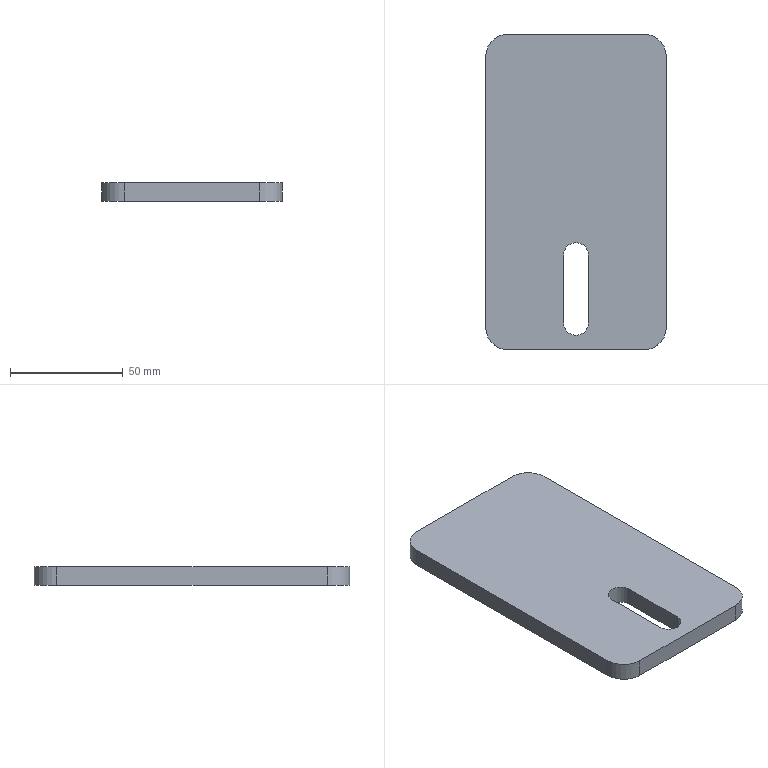Part | SolidWorks | features Extrusion 1, ICE 1 | 1 solid | 14 faces | box 80 x 140 x 8 mm | volume 85513 mm3 | plane 8 | cylinder 6 | commonest cylinder face diameters 20 x4 11 x2
STEP:
#1=CARTESIAN_POINT('',(70.,0.,0.));
#2=VERTEX_POINT('',#1);
#3=CARTESIAN_POINT('',(80.,10.,0.));
#4=VERTEX_POINT('',#3);
#5=CARTESIAN_POINT('',(70.,10.,0.));
#6=DIRECTION('',(0.,0.,1.));
#7=DIRECTION('',(-1.,0.,0.));
#8=AXIS2_PLACEMENT_3D('',#5,#6,#7);
#9=CIRCLE('',#8,10.);
#10=EDGE_CURVE('',#2,#4,#9,.T.);
#11=ORIENTED_EDGE('',*,*,#10,.T.);
#12=CARTESIAN_POINT('',(80.,10.,8.));
#13=VERTEX_POINT('',#12);
#14=CARTESIAN_POINT('',(80.,10.,8.));
#15=DIRECTION('',(0.,0.,-1.));
#16=VECTOR('',#15,1000.);
#17=LINE('',#14,#16);
#18=EDGE_CURVE('',#13,#4,#17,.T.);
#19=ORIENTED_EDGE('',*,*,#18,.F.);
#20=CARTESIAN_POINT('',(70.,0.,8.));
#21=VERTEX_POINT('',#20);
#22=CARTESIAN_POINT('',(70.,10.,8.));
#23=DIRECTION('',(0.,0.,1.));
#24=DIRECTION('',(-1.,0.,0.));
#25=AXIS2_PLACEMENT_3D('',#22,#23,#24);
#26=CIRCLE('',#25,10.);
#27=EDGE_CURVE('',#21,#13,#26,.T.);
#28=ORIENTED_EDGE('',*,*,#27,.F.);
#29=CARTESIAN_POINT('',(70.,0.,8.));
#30=DIRECTION('',(0.,0.,-1.));
#31=VECTOR('',#30,1000.);
#32=LINE('',#29,#31);
#33=EDGE_CURVE('',#21,#2,#32,.T.);
#34=ORIENTED_EDGE('',*,*,#33,.T.);
#35=EDGE_LOOP('',(#11,#19,#28,#34));
#36=FACE_OUTER_BOUND('',#35,.T.);
#37=CARTESIAN_POINT('',(70.,10.,8.));
#38=DIRECTION('',(0.,0.,-1.));
#39=DIRECTION('',(-1.,0.,0.));
#40=AXIS2_PLACEMENT_3D('',#37,#38,#39);
#41=CYLINDRICAL_SURFACE('',#40,10.);
#42=ADVANCED_FACE('',(#36),#41,.T.);
#43=CARTESIAN_POINT('',(80.,130.,0.));
#44=VERTEX_POINT('',#43);
#45=CARTESIAN_POINT('',(80.,10.,0.));
#46=DIRECTION('',(0.,1.,0.));
#47=VECTOR('',#46,1000.);
#48=LINE('',#45,#47);
#49=EDGE_CURVE('',#4,#44,#48,.T.);
#50=ORIENTED_EDGE('',*,*,#49,.T.);
#51=CARTESIAN_POINT('',(80.,130.,8.));
#52=VERTEX_POINT('',#51);
#53=CARTESIAN_POINT('',(80.,130.,8.));
#54=DIRECTION('',(0.,0.,-1.));
#55=VECTOR('',#54,1000.);
#56=LINE('',#53,#55);
#57=EDGE_CURVE('',#52,#44,#56,.T.);
#58=ORIENTED_EDGE('',*,*,#57,.F.);
#59=CARTESIAN_POINT('',(80.,10.,8.));
#60=DIRECTION('',(0.,1.,0.));
#61=VECTOR('',#60,1000.);
#62=LINE('',#59,#61);
#63=EDGE_CURVE('',#13,#52,#62,.T.);
#64=ORIENTED_EDGE('',*,*,#63,.F.);
#65=ORIENTED_EDGE('',*,*,#18,.T.);
#66=EDGE_LOOP('',(#50,#58,#64,#65));
#67=FACE_OUTER_BOUND('',#66,.T.);
#68=CARTESIAN_POINT('',(80.,10.,8.));
#69=DIRECTION('',(-1.,0.,0.));
#70=DIRECTION('',(0.,0.,1.));
#71=AXIS2_PLACEMENT_3D('',#68,#69,#70);
#72=PLANE('',#71);
#73=ADVANCED_FACE('',(#67),#72,.F.);
#74=CARTESIAN_POINT('',(70.,140.,0.));
#75=VERTEX_POINT('',#74);
#76=CARTESIAN_POINT('',(70.,130.,0.));
#77=DIRECTION('',(0.,0.,1.));
#78=DIRECTION('',(1.,0.,0.));
#79=AXIS2_PLACEMENT_3D('',#76,#77,#78);
#80=CIRCLE('',#79,10.);
#81=EDGE_CURVE('',#44,#75,#80,.T.);
#82=ORIENTED_EDGE('',*,*,#81,.T.);
#83=CARTESIAN_POINT('',(70.,140.,8.));
#84=VERTEX_POINT('',#83);
#85=CARTESIAN_POINT('',(70.,140.,8.));
#86=DIRECTION('',(0.,0.,-1.));
#87=VECTOR('',#86,1000.);
#88=LINE('',#85,#87);
#89=EDGE_CURVE('',#84,#75,#88,.T.);
#90=ORIENTED_EDGE('',*,*,#89,.F.);
#91=CARTESIAN_POINT('',(70.,130.,8.));
#92=DIRECTION('',(0.,0.,1.));
#93=DIRECTION('',(1.,0.,0.));
#94=AXIS2_PLACEMENT_3D('',#91,#92,#93);
#95=CIRCLE('',#94,10.);
#96=EDGE_CURVE('',#52,#84,#95,.T.);
#97=ORIENTED_EDGE('',*,*,#96,.F.);
#98=ORIENTED_EDGE('',*,*,#57,.T.);
#99=EDGE_LOOP('',(#82,#90,#97,#98));
#100=FACE_OUTER_BOUND('',#99,.T.);
#101=CARTESIAN_POINT('',(70.,130.,8.));
#102=DIRECTION('',(0.,0.,-1.));
#103=DIRECTION('',(-1.,0.,0.));
#104=AXIS2_PLACEMENT_3D('',#101,#102,#103);
#105=CYLINDRICAL_SURFACE('',#104,10.);
#106=ADVANCED_FACE('',(#100),#105,.T.);
#107=CARTESIAN_POINT('',(10.,140.,0.));
#108=VERTEX_POINT('',#107);
#109=CARTESIAN_POINT('',(10.,140.,0.));
#110=DIRECTION('',(-1.,0.,0.));
#111=VECTOR('',#110,1000.);
#112=LINE('',#109,#111);
#113=EDGE_CURVE('',#75,#108,#112,.T.);
#114=ORIENTED_EDGE('',*,*,#113,.T.);
#115=CARTESIAN_POINT('',(10.,140.,8.));
#116=VERTEX_POINT('',#115);
#117=CARTESIAN_POINT('',(10.,140.,8.));
#118=DIRECTION('',(0.,0.,-1.));
#119=VECTOR('',#118,1000.);
#120=LINE('',#117,#119);
#121=EDGE_CURVE('',#116,#108,#120,.T.);
#122=ORIENTED_EDGE('',*,*,#121,.F.);
#123=CARTESIAN_POINT('',(10.,140.,8.));
#124=DIRECTION('',(-1.,0.,0.));
#125=VECTOR('',#124,1000.);
#126=LINE('',#123,#125);
#127=EDGE_CURVE('',#84,#116,#126,.T.);
#128=ORIENTED_EDGE('',*,*,#127,.F.);
#129=ORIENTED_EDGE('',*,*,#89,.T.);
#130=EDGE_LOOP('',(#114,#122,#128,#129));
#131=FACE_OUTER_BOUND('',#130,.T.);
#132=CARTESIAN_POINT('',(10.,140.,8.));
#133=DIRECTION('',(0.,-1.,0.));
#134=DIRECTION('',(0.,0.,-1.));
#135=AXIS2_PLACEMENT_3D('',#132,#133,#134);
#136=PLANE('',#135);
#137=ADVANCED_FACE('',(#131),#136,.F.);
#138=CARTESIAN_POINT('',(0.,130.,0.));
#139=VERTEX_POINT('',#138);
#140=CARTESIAN_POINT('',(10.,130.,0.));
#141=DIRECTION('',(0.,0.,1.));
#142=DIRECTION('',(-1.,0.,0.));
#143=AXIS2_PLACEMENT_3D('',#140,#141,#142);
#144=CIRCLE('',#143,10.);
#145=EDGE_CURVE('',#108,#139,#144,.T.);
#146=ORIENTED_EDGE('',*,*,#145,.T.);
#147=CARTESIAN_POINT('',(0.,130.,8.));
#148=VERTEX_POINT('',#147);
#149=CARTESIAN_POINT('',(0.,130.,8.));
#150=DIRECTION('',(0.,0.,-1.));
#151=VECTOR('',#150,1000.);
#152=LINE('',#149,#151);
#153=EDGE_CURVE('',#148,#139,#152,.T.);
#154=ORIENTED_EDGE('',*,*,#153,.F.);
#155=CARTESIAN_POINT('',(10.,130.,8.));
#156=DIRECTION('',(0.,0.,1.));
#157=DIRECTION('',(-1.,0.,0.));
#158=AXIS2_PLACEMENT_3D('',#155,#156,#157);
#159=CIRCLE('',#158,10.);
#160=EDGE_CURVE('',#116,#148,#159,.T.);
#161=ORIENTED_EDGE('',*,*,#160,.F.);
#162=ORIENTED_EDGE('',*,*,#121,.T.);
#163=EDGE_LOOP('',(#146,#154,#161,#162));
#164=FACE_OUTER_BOUND('',#163,.T.);
#165=CARTESIAN_POINT('',(10.,130.,8.));
#166=DIRECTION('',(0.,0.,-1.));
#167=DIRECTION('',(-1.,0.,0.));
#168=AXIS2_PLACEMENT_3D('',#165,#166,#167);
#169=CYLINDRICAL_SURFACE('',#168,10.);
#170=ADVANCED_FACE('',(#164),#169,.T.);
#171=CARTESIAN_POINT('',(0.,10.,0.));
#172=VERTEX_POINT('',#171);
#173=CARTESIAN_POINT('',(0.,10.,0.));
#174=DIRECTION('',(0.,-1.,0.));
#175=VECTOR('',#174,1000.);
#176=LINE('',#173,#175);
#177=EDGE_CURVE('',#139,#172,#176,.T.);
#178=ORIENTED_EDGE('',*,*,#177,.T.);
#179=CARTESIAN_POINT('',(0.,10.,8.));
#180=VERTEX_POINT('',#179);
#181=CARTESIAN_POINT('',(0.,10.,8.));
#182=DIRECTION('',(0.,0.,-1.));
#183=VECTOR('',#182,1000.);
#184=LINE('',#181,#183);
#185=EDGE_CURVE('',#180,#172,#184,.T.);
#186=ORIENTED_EDGE('',*,*,#185,.F.);
#187=CARTESIAN_POINT('',(0.,10.,8.));
#188=DIRECTION('',(0.,-1.,0.));
#189=VECTOR('',#188,1000.);
#190=LINE('',#187,#189);
#191=EDGE_CURVE('',#148,#180,#190,.T.);
#192=ORIENTED_EDGE('',*,*,#191,.F.);
#193=ORIENTED_EDGE('',*,*,#153,.T.);
#194=EDGE_LOOP('',(#178,#186,#192,#193));
#195=FACE_OUTER_BOUND('',#194,.T.);
#196=CARTESIAN_POINT('',(0.,10.,8.));
#197=DIRECTION('',(1.,0.,0.));
#198=DIRECTION('',(0.,0.,-1.));
#199=AXIS2_PLACEMENT_3D('',#196,#197,#198);
#200=PLANE('',#199);
#201=ADVANCED_FACE('',(#195),#200,.F.);
#202=CARTESIAN_POINT('',(10.,0.,0.));
#203=VERTEX_POINT('',#202);
#204=CARTESIAN_POINT('',(10.,10.,0.));
#205=DIRECTION('',(0.,0.,1.));
#206=DIRECTION('',(-1.,0.,0.));
#207=AXIS2_PLACEMENT_3D('',#204,#205,#206);
#208=CIRCLE('',#207,10.);
#209=EDGE_CURVE('',#172,#203,#208,.T.);
#210=ORIENTED_EDGE('',*,*,#209,.T.);
#211=CARTESIAN_POINT('',(10.,0.,8.));
#212=VERTEX_POINT('',#211);
#213=CARTESIAN_POINT('',(10.,0.,8.));
#214=DIRECTION('',(0.,0.,-1.));
#215=VECTOR('',#214,1000.);
#216=LINE('',#213,#215);
#217=EDGE_CURVE('',#212,#203,#216,.T.);
#218=ORIENTED_EDGE('',*,*,#217,.F.);
#219=CARTESIAN_POINT('',(10.,10.,8.));
#220=DIRECTION('',(0.,0.,1.));
#221=DIRECTION('',(-1.,0.,0.));
#222=AXIS2_PLACEMENT_3D('',#219,#220,#221);
#223=CIRCLE('',#222,10.);
#224=EDGE_CURVE('',#180,#212,#223,.T.);
#225=ORIENTED_EDGE('',*,*,#224,.F.);
#226=ORIENTED_EDGE('',*,*,#185,.T.);
#227=EDGE_LOOP('',(#210,#218,#225,#226));
#228=FACE_OUTER_BOUND('',#227,.T.);
#229=CARTESIAN_POINT('',(10.,10.,8.));
#230=DIRECTION('',(0.,0.,-1.));
#231=DIRECTION('',(-1.,0.,0.));
#232=AXIS2_PLACEMENT_3D('',#229,#230,#231);
#233=CYLINDRICAL_SURFACE('',#232,10.);
#234=ADVANCED_FACE('',(#228),#233,.T.);
#235=CARTESIAN_POINT('',(10.,0.,0.));
#236=DIRECTION('',(1.,0.,0.));
#237=VECTOR('',#236,1000.);
#238=LINE('',#235,#237);
#239=EDGE_CURVE('',#203,#2,#238,.T.);
#240=ORIENTED_EDGE('',*,*,#239,.T.);
#241=ORIENTED_EDGE('',*,*,#33,.F.);
#242=CARTESIAN_POINT('',(10.,0.,8.));
#243=DIRECTION('',(1.,0.,0.));
#244=VECTOR('',#243,1000.);
#245=LINE('',#242,#244);
#246=EDGE_CURVE('',#212,#21,#245,.T.);
#247=ORIENTED_EDGE('',*,*,#246,.F.);
#248=ORIENTED_EDGE('',*,*,#217,.T.);
#249=EDGE_LOOP('',(#240,#241,#247,#248));
#250=FACE_OUTER_BOUND('',#249,.T.);
#251=CARTESIAN_POINT('',(10.,0.,8.));
#252=DIRECTION('',(0.,1.,0.));
#253=DIRECTION('',(0.,0.,1.));
#254=AXIS2_PLACEMENT_3D('',#251,#252,#253);
#255=PLANE('',#254);
#256=ADVANCED_FACE('',(#250),#255,.F.);
#257=CARTESIAN_POINT('',(45.5,12.,8.));
#258=VERTEX_POINT('',#257);
#259=CARTESIAN_POINT('',(45.5,42.,8.));
#260=VERTEX_POINT('',#259);
#261=CARTESIAN_POINT('',(45.5,12.,8.));
#262=DIRECTION('',(0.,1.,0.));
#263=VECTOR('',#262,1000.);
#264=LINE('',#261,#263);
#265=EDGE_CURVE('',#258,#260,#264,.T.);
#266=ORIENTED_EDGE('',*,*,#265,.F.);
#267=CARTESIAN_POINT('',(34.5,12.,8.));
#268=VERTEX_POINT('',#267);
#269=CARTESIAN_POINT('',(40.,12.,8.));
#270=DIRECTION('',(0.,0.,1.));
#271=DIRECTION('',(1.,0.,0.));
#272=AXIS2_PLACEMENT_3D('',#269,#270,#271);
#273=CIRCLE('',#272,5.5);
#274=EDGE_CURVE('',#268,#258,#273,.T.);
#275=ORIENTED_EDGE('',*,*,#274,.F.);
#276=CARTESIAN_POINT('',(34.5,42.,8.));
#277=VERTEX_POINT('',#276);
#278=CARTESIAN_POINT('',(34.5,12.,8.));
#279=DIRECTION('',(0.,-1.,0.));
#280=VECTOR('',#279,1000.);
#281=LINE('',#278,#280);
#282=EDGE_CURVE('',#277,#268,#281,.T.);
#283=ORIENTED_EDGE('',*,*,#282,.F.);
#284=CARTESIAN_POINT('',(40.,42.,8.));
#285=DIRECTION('',(0.,0.,1.));
#286=DIRECTION('',(1.,0.,0.));
#287=AXIS2_PLACEMENT_3D('',#284,#285,#286);
#288=CIRCLE('',#287,5.5);
#289=EDGE_CURVE('',#260,#277,#288,.T.);
#290=ORIENTED_EDGE('',*,*,#289,.F.);
#291=EDGE_LOOP('',(#266,#275,#283,#290));
#292=FACE_BOUND('',#291,.T.);
#293=ORIENTED_EDGE('',*,*,#27,.T.);
#294=ORIENTED_EDGE('',*,*,#63,.T.);
#295=ORIENTED_EDGE('',*,*,#96,.T.);
#296=ORIENTED_EDGE('',*,*,#127,.T.);
#297=ORIENTED_EDGE('',*,*,#160,.T.);
#298=ORIENTED_EDGE('',*,*,#191,.T.);
#299=ORIENTED_EDGE('',*,*,#224,.T.);
#300=ORIENTED_EDGE('',*,*,#246,.T.);
#301=EDGE_LOOP('',(#293,#294,#295,#296,#297,#298,#299,#300));
#302=FACE_OUTER_BOUND('',#301,.T.);
#303=CARTESIAN_POINT('',(70.,10.,8.));
#304=DIRECTION('',(0.,0.,-1.));
#305=DIRECTION('',(-1.,0.,0.));
#306=AXIS2_PLACEMENT_3D('',#303,#304,#305);
#307=PLANE('',#306);
#308=ADVANCED_FACE('',(#292,#302),#307,.F.);
#309=CARTESIAN_POINT('',(45.5,12.,0.));
#310=VERTEX_POINT('',#309);
#311=CARTESIAN_POINT('',(34.5,12.,0.));
#312=VERTEX_POINT('',#311);
#313=CARTESIAN_POINT('',(40.,12.,0.));
#314=DIRECTION('',(0.,0.,-1.));
#315=DIRECTION('',(-1.,0.,0.));
#316=AXIS2_PLACEMENT_3D('',#313,#314,#315);
#317=CIRCLE('',#316,5.5);
#318=EDGE_CURVE('',#310,#312,#317,.T.);
#319=ORIENTED_EDGE('',*,*,#318,.F.);
#320=CARTESIAN_POINT('',(45.5,42.,0.));
#321=VERTEX_POINT('',#320);
#322=CARTESIAN_POINT('',(45.5,10.,0.));
#323=DIRECTION('',(0.,-1.,0.));
#324=VECTOR('',#323,1000.);
#325=LINE('',#322,#324);
#326=EDGE_CURVE('',#321,#310,#325,.T.);
#327=ORIENTED_EDGE('',*,*,#326,.F.);
#328=CARTESIAN_POINT('',(34.5,42.,0.));
#329=VERTEX_POINT('',#328);
#330=CARTESIAN_POINT('',(40.,42.,0.));
#331=DIRECTION('',(0.,0.,-1.));
#332=DIRECTION('',(-1.,0.,0.));
#333=AXIS2_PLACEMENT_3D('',#330,#331,#332);
#334=CIRCLE('',#333,5.5);
#335=EDGE_CURVE('',#329,#321,#334,.T.);
#336=ORIENTED_EDGE('',*,*,#335,.F.);
#337=CARTESIAN_POINT('',(34.5,10.,0.));
#338=DIRECTION('',(0.,1.,0.));
#339=VECTOR('',#338,1000.);
#340=LINE('',#337,#339);
#341=EDGE_CURVE('',#312,#329,#340,.T.);
#342=ORIENTED_EDGE('',*,*,#341,.F.);
#343=EDGE_LOOP('',(#319,#327,#336,#342));
#344=FACE_BOUND('',#343,.T.);
#345=ORIENTED_EDGE('',*,*,#10,.F.);
#346=ORIENTED_EDGE('',*,*,#239,.F.);
#347=ORIENTED_EDGE('',*,*,#209,.F.);
#348=ORIENTED_EDGE('',*,*,#177,.F.);
#349=ORIENTED_EDGE('',*,*,#145,.F.);
#350=ORIENTED_EDGE('',*,*,#113,.F.);
#351=ORIENTED_EDGE('',*,*,#81,.F.);
#352=ORIENTED_EDGE('',*,*,#49,.F.);
#353=EDGE_LOOP('',(#345,#346,#347,#348,#349,#350,#351,#352));
#354=FACE_OUTER_BOUND('',#353,.T.);
#355=CARTESIAN_POINT('',(70.,10.,0.));
#356=DIRECTION('',(0.,0.,-1.));
#357=DIRECTION('',(-1.,0.,0.));
#358=AXIS2_PLACEMENT_3D('',#355,#356,#357);
#359=PLANE('',#358);
#360=ADVANCED_FACE('',(#344,#354),#359,.T.);
#361=ORIENTED_EDGE('',*,*,#318,.T.);
#362=CARTESIAN_POINT('',(34.5,12.,-2.));
#363=DIRECTION('',(0.,0.,1.));
#364=VECTOR('',#363,1000.);
#365=LINE('',#362,#364);
#366=EDGE_CURVE('',#312,#268,#365,.T.);
#367=ORIENTED_EDGE('',*,*,#366,.T.);
#368=ORIENTED_EDGE('',*,*,#274,.T.);
#369=CARTESIAN_POINT('',(45.5,12.,-2.));
#370=DIRECTION('',(0.,0.,1.));
#371=VECTOR('',#370,1000.);
#372=LINE('',#369,#371);
#373=EDGE_CURVE('',#310,#258,#372,.T.);
#374=ORIENTED_EDGE('',*,*,#373,.F.);
#375=EDGE_LOOP('',(#361,#367,#368,#374));
#376=FACE_OUTER_BOUND('',#375,.T.);
#377=CARTESIAN_POINT('',(40.,12.,-2.));
#378=DIRECTION('',(0.,0.,1.));
#379=DIRECTION('',(1.,0.,0.));
#380=AXIS2_PLACEMENT_3D('',#377,#378,#379);
#381=CYLINDRICAL_SURFACE('',#380,5.5);
#382=ADVANCED_FACE('',(#376),#381,.F.);
#383=ORIENTED_EDGE('',*,*,#341,.T.);
#384=CARTESIAN_POINT('',(34.5,42.,-2.));
#385=DIRECTION('',(0.,0.,1.));
#386=VECTOR('',#385,1000.);
#387=LINE('',#384,#386);
#388=EDGE_CURVE('',#329,#277,#387,.T.);
#389=ORIENTED_EDGE('',*,*,#388,.T.);
#390=ORIENTED_EDGE('',*,*,#282,.T.);
#391=ORIENTED_EDGE('',*,*,#366,.F.);
#392=EDGE_LOOP('',(#383,#389,#390,#391));
#393=FACE_OUTER_BOUND('',#392,.T.);
#394=CARTESIAN_POINT('',(34.5,12.,-2.));
#395=DIRECTION('',(-1.,0.,0.));
#396=DIRECTION('',(0.,-1.,0.));
#397=AXIS2_PLACEMENT_3D('',#394,#395,#396);
#398=PLANE('',#397);
#399=ADVANCED_FACE('',(#393),#398,.F.);
#400=ORIENTED_EDGE('',*,*,#335,.T.);
#401=CARTESIAN_POINT('',(45.5,42.,-2.));
#402=DIRECTION('',(0.,0.,1.));
#403=VECTOR('',#402,1000.);
#404=LINE('',#401,#403);
#405=EDGE_CURVE('',#321,#260,#404,.T.);
#406=ORIENTED_EDGE('',*,*,#405,.T.);
#407=ORIENTED_EDGE('',*,*,#289,.T.);
#408=ORIENTED_EDGE('',*,*,#388,.F.);
#409=EDGE_LOOP('',(#400,#406,#407,#408));
#410=FACE_OUTER_BOUND('',#409,.T.);
#411=CARTESIAN_POINT('',(40.,42.,-2.));
#412=DIRECTION('',(0.,0.,1.));
#413=DIRECTION('',(1.,0.,0.));
#414=AXIS2_PLACEMENT_3D('',#411,#412,#413);
#415=CYLINDRICAL_SURFACE('',#414,5.5);
#416=ADVANCED_FACE('',(#410),#415,.F.);
#417=ORIENTED_EDGE('',*,*,#326,.T.);
#418=ORIENTED_EDGE('',*,*,#373,.T.);
#419=ORIENTED_EDGE('',*,*,#265,.T.);
#420=ORIENTED_EDGE('',*,*,#405,.F.);
#421=EDGE_LOOP('',(#417,#418,#419,#420));
#422=FACE_OUTER_BOUND('',#421,.T.);
#423=CARTESIAN_POINT('',(45.5,12.,-2.));
#424=DIRECTION('',(1.,0.,0.));
#425=DIRECTION('',(0.,1.,0.));
#426=AXIS2_PLACEMENT_3D('',#423,#424,#425);
#427=PLANE('',#426);
#428=ADVANCED_FACE('',(#422),#427,.F.);
#429=CLOSED_SHELL('',(#42,#73,#106,#137,#170,#201,#234,#256,#308,#360,#382,#399,#416,#428));
#430=MANIFOLD_SOLID_BREP('',#429);
#431=CARTESIAN_POINT('',(0.,0.,0.));
#432=DIRECTION('',(0.,0.,1.));
#433=DIRECTION('',(1.,0.,0.));
#434=AXIS2_PLACEMENT_3D('',#431,#432,#433);
#435=(LENGTH_UNIT()NAMED_UNIT(*)SI_UNIT(.MILLI.,.METRE.));
#436=UNCERTAINTY_MEASURE_WITH_UNIT(LENGTH_MEASURE(0.00001),#435,'','');
#437=(NAMED_UNIT(*)PLANE_ANGLE_UNIT()SI_UNIT($,.RADIAN.));
#438=(NAMED_UNIT(*)SI_UNIT($,.STERADIAN.)SOLID_ANGLE_UNIT());
#439=(GEOMETRIC_REPRESENTATION_CONTEXT(3)GLOBAL_UNCERTAINTY_ASSIGNED_CONTEXT((#436))GLOBAL_UNIT_ASSIGNED_CONTEXT((#435,#437,#438))REPRESENTATION_CONTEXT('',''));
#440=ADVANCED_BREP_SHAPE_REPRESENTATION('',(#430,#434),#439);